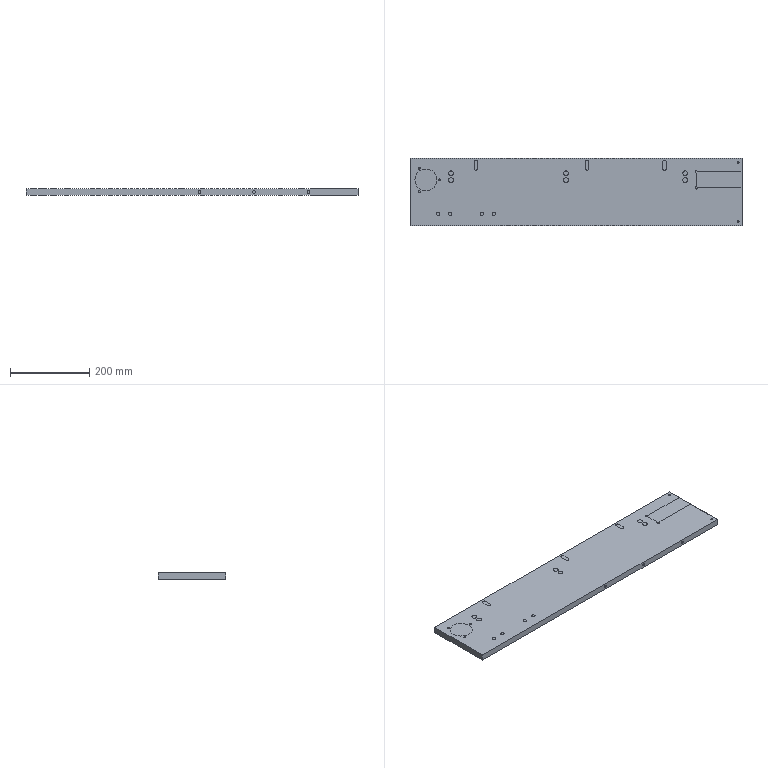NC program | NX | posted with a generic post | part box 836 x 170 x 16 mm
Lines 11488 to 11551 of 11551:
(2D边界补正 , TOOL : D10平底刀)
N22950 T06 M6
N22952 /M1
N22954 G54
N22956 G17 G0 G90 X23.271 Y116.575 S3000 M3
N22958 G43 Z100. H6
N22960 Z-16.
N22962 G94 G1 Z-17. F400.
N22964 G41 X23.219 Y116.768 D6
N22966 G3 X17.5 Y115.5 R3.
N22968 X40. Y93. R22.5 F500.
N22970 X17.5 Y115.5 R-22.5
N22972 G1 X17.501 Y115.3
N22974 G3 X23.231 Y114.083 R3.
N22976 G40
N22978 G1 X23.281 Y114.277
N22980 Z-16.
N22982 G0 Z100.
(G81点孔_1 , TOOL : D6点孔钻)
N22984 T01 M6
N22986 /M1
N22988 G17 G43 G0 G90 X103. Y132. Z100. S1500 H1 M3
N22990 G94 G81 G98 Z-8.5 F60. R-5.5
N22992 Y115.
N22994 X393. Y132.
N22996 Y115.
N22998 X693. Y132.
N23000 Y115.
N23002 G80
N23004 G0 X693. Y115. Z100.
N23006 M5
(边界倒角_1 , TOOL : D6倒角刀)
N23008 T07 M6
N23010 /M1
N23012 G54
N23014 G17 G0 G90 X837. Y130.7 S3000 M3
N23016 G43 Z100. H7
N23018 Z-1.5
N23020 G94 G1 Z-2.5 F640.
N23022 G3 X836. Y131.7 R1.
N23024 G1 X724.8 F800.
N23026 Y99.3
N23028 X836.
N23030 G3 X837. Y100.3 R1.
N23032 G1 Z-1.5
N23034 G0 Z100.
N23036 X17.3 Y116.5
N23038 Z-1.5
N23040 G1 Z-2.5 F640.
N23042 G3 X16.3 Y115.5 R1.
N23044 X40. Y91.8 R23.7 F800.
N23046 X16.3 Y115.5 R-23.7
N23048 G1 X16.301 Y115.3
N23050 G3 X17.309 Y114.308 R1.
N23052 G1 Z-1.5
N23054 G0 Z100.
N23056 M5
N23058 M2